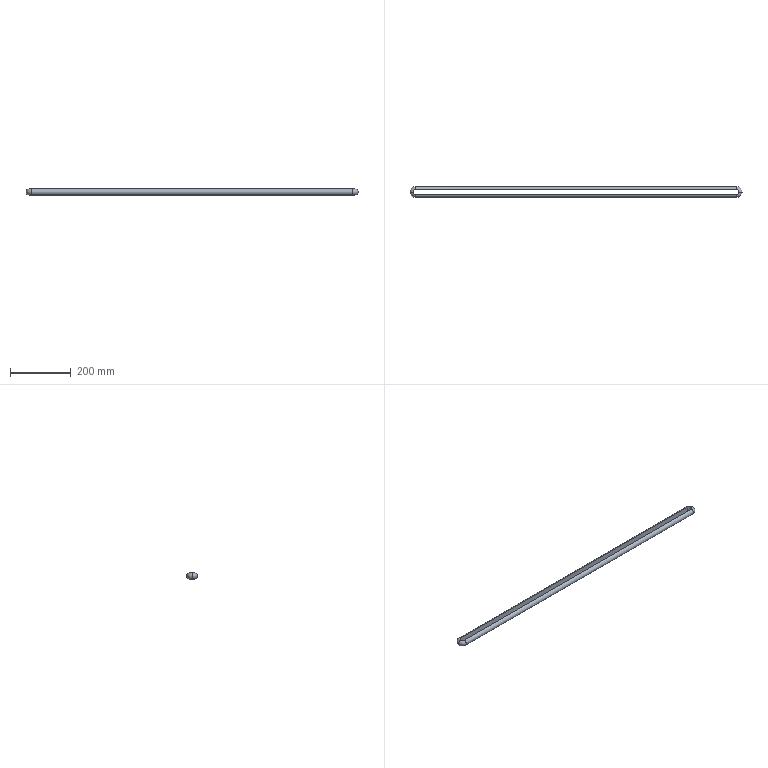Part | SolidWorks | features Sweep 1 | 1 solid | 11 faces | box 1096 x 36 x 20 mm | volume 345093 mm3 | cylinder 5 | torus 4 | plane 2 | commonest cylinder face diameters 16 x3 20 x2
STEP:
#1=CARTESIAN_POINT('',(1060.,8.,10.));
#2=VERTEX_POINT('',#1);
#3=CARTESIAN_POINT('',(1068.,0.,10.));
#4=VERTEX_POINT('',#3);
#5=CARTESIAN_POINT('',(1060.,0.,10.));
#6=DIRECTION('',(0.,0.,-1.));
#7=DIRECTION('',(-1.,0.,0.));
#8=AXIS2_PLACEMENT_3D('',#5,#6,#7);
#9=CIRCLE('',#8,8.);
#10=EDGE_CURVE('',#2,#4,#9,.T.);
#11=ORIENTED_EDGE('',*,*,#10,.T.);
#12=CARTESIAN_POINT('',(1068.,0.,-10.));
#13=VERTEX_POINT('',#12);
#14=CARTESIAN_POINT('',(1068.,0.,0.));
#15=DIRECTION('',(0.,1.,0.));
#16=DIRECTION('',(-1.,0.,0.));
#17=AXIS2_PLACEMENT_3D('',#14,#15,#16);
#18=CIRCLE('',#17,10.);
#19=EDGE_CURVE('',#4,#13,#18,.T.);
#20=ORIENTED_EDGE('',*,*,#19,.T.);
#21=CARTESIAN_POINT('',(1060.,8.,-10.));
#22=VERTEX_POINT('',#21);
#23=CARTESIAN_POINT('',(1060.,0.,-10.));
#24=DIRECTION('',(0.,0.,-1.));
#25=DIRECTION('',(-1.,0.,0.));
#26=AXIS2_PLACEMENT_3D('',#23,#24,#25);
#27=CIRCLE('',#26,8.);
#28=EDGE_CURVE('',#22,#13,#27,.T.);
#29=ORIENTED_EDGE('',*,*,#28,.F.);
#30=CARTESIAN_POINT('',(1060.,8.,0.));
#31=DIRECTION('',(1.,0.,0.));
#32=DIRECTION('',(0.,0.,-1.));
#33=AXIS2_PLACEMENT_3D('',#30,#31,#32);
#34=CIRCLE('',#33,10.);
#35=EDGE_CURVE('',#22,#2,#34,.T.);
#36=ORIENTED_EDGE('',*,*,#35,.T.);
#37=EDGE_LOOP('',(#11,#20,#29,#36));
#38=FACE_OUTER_BOUND('',#37,.T.);
#39=CARTESIAN_POINT('',(1060.,0.,0.));
#40=DIRECTION('',(0.,0.,-1.));
#41=DIRECTION('',(-1.,0.,0.));
#42=AXIS2_PLACEMENT_3D('',#39,#40,#41);
#43=TOROIDAL_SURFACE('',#42,8.,10.);
#44=ADVANCED_FACE('',(#38),#43,.T.);
#45=CARTESIAN_POINT('',(0.,-8.,10.));
#46=VERTEX_POINT('',#45);
#47=CARTESIAN_POINT('',(-8.,0.,10.));
#48=VERTEX_POINT('',#47);
#49=CARTESIAN_POINT('',(0.,0.,10.));
#50=DIRECTION('',(0.,0.,-1.));
#51=DIRECTION('',(-1.,0.,0.));
#52=AXIS2_PLACEMENT_3D('',#49,#50,#51);
#53=CIRCLE('',#52,8.);
#54=EDGE_CURVE('',#46,#48,#53,.T.);
#55=ORIENTED_EDGE('',*,*,#54,.T.);
#56=CARTESIAN_POINT('',(-8.,0.,-10.));
#57=VERTEX_POINT('',#56);
#58=CARTESIAN_POINT('',(-8.,0.,0.));
#59=DIRECTION('',(0.,-1.,0.));
#60=DIRECTION('',(0.,0.,-1.));
#61=AXIS2_PLACEMENT_3D('',#58,#59,#60);
#62=CIRCLE('',#61,10.);
#63=EDGE_CURVE('',#48,#57,#62,.T.);
#64=ORIENTED_EDGE('',*,*,#63,.T.);
#65=CARTESIAN_POINT('',(0.,-8.,-10.));
#66=VERTEX_POINT('',#65);
#67=CARTESIAN_POINT('',(0.,0.,-10.));
#68=DIRECTION('',(0.,0.,-1.));
#69=DIRECTION('',(-1.,0.,0.));
#70=AXIS2_PLACEMENT_3D('',#67,#68,#69);
#71=CIRCLE('',#70,8.);
#72=EDGE_CURVE('',#66,#57,#71,.T.);
#73=ORIENTED_EDGE('',*,*,#72,.F.);
#74=CARTESIAN_POINT('',(0.,-8.,0.));
#75=DIRECTION('',(-1.,0.,0.));
#76=DIRECTION('',(0.,0.,-1.));
#77=AXIS2_PLACEMENT_3D('',#74,#75,#76);
#78=CIRCLE('',#77,10.);
#79=EDGE_CURVE('',#66,#46,#78,.T.);
#80=ORIENTED_EDGE('',*,*,#79,.T.);
#81=EDGE_LOOP('',(#55,#64,#73,#80));
#82=FACE_OUTER_BOUND('',#81,.T.);
#83=CARTESIAN_POINT('',(0.,0.,0.));
#84=DIRECTION('',(0.,0.,-1.));
#85=DIRECTION('',(-1.,0.,0.));
#86=AXIS2_PLACEMENT_3D('',#83,#84,#85);
#87=TOROIDAL_SURFACE('',#86,8.,10.);
#88=ADVANCED_FACE('',(#82),#87,.T.);
#89=CARTESIAN_POINT('',(0.,8.,10.));
#90=VERTEX_POINT('',#89);
#91=CARTESIAN_POINT('',(0.,0.,10.));
#92=DIRECTION('',(0.,0.,-1.));
#93=DIRECTION('',(-1.,0.,0.));
#94=AXIS2_PLACEMENT_3D('',#91,#92,#93);
#95=CIRCLE('',#94,8.);
#96=EDGE_CURVE('',#48,#90,#95,.T.);
#97=ORIENTED_EDGE('',*,*,#96,.F.);
#98=CARTESIAN_POINT('',(-8.,0.,0.));
#99=DIRECTION('',(0.,0.,-1.));
#100=VECTOR('',#99,1000.);
#101=LINE('',#98,#100);
#102=EDGE_CURVE('',#48,#57,#101,.T.);
#103=ORIENTED_EDGE('',*,*,#102,.T.);
#104=CARTESIAN_POINT('',(0.,8.,-10.));
#105=VERTEX_POINT('',#104);
#106=CARTESIAN_POINT('',(0.,0.,-10.));
#107=DIRECTION('',(0.,0.,-1.));
#108=DIRECTION('',(-1.,0.,0.));
#109=AXIS2_PLACEMENT_3D('',#106,#107,#108);
#110=CIRCLE('',#109,8.);
#111=EDGE_CURVE('',#57,#105,#110,.T.);
#112=ORIENTED_EDGE('',*,*,#111,.T.);
#113=CARTESIAN_POINT('',(0.,8.,10.));
#114=CARTESIAN_POINT('',(0.,8.,3.333));
#115=CARTESIAN_POINT('',(0.,8.,-3.333));
#116=CARTESIAN_POINT('',(0.,8.,-10.));
#117=B_SPLINE_CURVE_WITH_KNOTS('',3,(#113,#114,#115,#116),.UNSPECIFIED.,.F.,.F.,(4,4),(0.,1.),.UNSPECIFIED.);
#118=EDGE_CURVE('',#90,#105,#117,.T.);
#119=ORIENTED_EDGE('',*,*,#118,.F.);
#120=EDGE_LOOP('',(#97,#103,#112,#119));
#121=FACE_OUTER_BOUND('',#120,.T.);
#122=CARTESIAN_POINT('',(0.,0.,0.));
#123=DIRECTION('',(0.,0.,-1.));
#124=DIRECTION('',(-1.,0.,0.));
#125=AXIS2_PLACEMENT_3D('',#122,#123,#124);
#126=CYLINDRICAL_SURFACE('',#125,8.);
#127=ADVANCED_FACE('',(#121),#126,.F.);
#128=ORIENTED_EDGE('',*,*,#102,.F.);
#129=ORIENTED_EDGE('',*,*,#54,.F.);
#130=CARTESIAN_POINT('',(0.,-8.,10.));
#131=DIRECTION('',(0.,0.,-1.));
#132=VECTOR('',#131,1000.);
#133=LINE('',#130,#132);
#134=EDGE_CURVE('',#46,#66,#133,.T.);
#135=ORIENTED_EDGE('',*,*,#134,.T.);
#136=ORIENTED_EDGE('',*,*,#72,.T.);
#137=EDGE_LOOP('',(#128,#129,#135,#136));
#138=FACE_OUTER_BOUND('',#137,.T.);
#139=CARTESIAN_POINT('',(0.,0.,0.));
#140=DIRECTION('',(0.,0.,-1.));
#141=DIRECTION('',(-1.,0.,0.));
#142=AXIS2_PLACEMENT_3D('',#139,#140,#141);
#143=CYLINDRICAL_SURFACE('',#142,8.);
#144=ADVANCED_FACE('',(#138),#143,.F.);
#145=ORIENTED_EDGE('',*,*,#63,.F.);
#146=ORIENTED_EDGE('',*,*,#96,.T.);
#147=CARTESIAN_POINT('',(0.,8.,-10.));
#148=CARTESIAN_POINT('',(0.,9.309,-10.));
#149=CARTESIAN_POINT('',(0.,10.617,-9.74));
#150=CARTESIAN_POINT('',(0.,13.036,-8.738));
#151=CARTESIAN_POINT('',(0.,14.145,-7.997));
#152=CARTESIAN_POINT('',(0.,15.997,-6.145));
#153=CARTESIAN_POINT('',(0.,16.738,-5.036));
#154=CARTESIAN_POINT('',(0.,17.74,-2.617));
#155=CARTESIAN_POINT('',(0.,18.,-1.309));
#156=CARTESIAN_POINT('',(0.,18.,1.309));
#157=CARTESIAN_POINT('',(0.,17.74,2.617));
#158=CARTESIAN_POINT('',(0.,16.738,5.036));
#159=CARTESIAN_POINT('',(0.,15.997,6.145));
#160=CARTESIAN_POINT('',(0.,14.145,7.997));
#161=CARTESIAN_POINT('',(0.,13.036,8.738));
#162=CARTESIAN_POINT('',(0.,10.617,9.74));
#163=CARTESIAN_POINT('',(0.,9.309,10.));
#164=CARTESIAN_POINT('',(0.,8.,10.));
#165=B_SPLINE_CURVE_WITH_KNOTS('',3,(#147,#148,#149,#150,#151,#152,#153,#154,#155,#156,#157,#158,#159,#160,#161,#162,#163,#164),.UNSPECIFIED.,.F.,.F.,(4,2,2,2,2,2,2,2,4),(0.,0.125,0.25,0.375,0.5,0.625,0.75,0.875,1.),.UNSPECIFIED.);
#166=EDGE_CURVE('',#105,#90,#165,.T.);
#167=ORIENTED_EDGE('',*,*,#166,.F.);
#168=ORIENTED_EDGE('',*,*,#111,.F.);
#169=EDGE_LOOP('',(#145,#146,#167,#168));
#170=FACE_OUTER_BOUND('',#169,.T.);
#171=CARTESIAN_POINT('',(0.,0.,0.));
#172=DIRECTION('',(0.,0.,-1.));
#173=DIRECTION('',(-1.,0.,0.));
#174=AXIS2_PLACEMENT_3D('',#171,#172,#173);
#175=TOROIDAL_SURFACE('',#174,8.,10.);
#176=ADVANCED_FACE('',(#170),#175,.T.);
#177=CARTESIAN_POINT('',(1060.,-8.,10.));
#178=VERTEX_POINT('',#177);
#179=CARTESIAN_POINT('',(1060.,-8.,-10.));
#180=VERTEX_POINT('',#179);
#181=CARTESIAN_POINT('',(1060.,-8.,10.));
#182=DIRECTION('',(0.,0.,-1.));
#183=VECTOR('',#182,1000.);
#184=LINE('',#181,#183);
#185=EDGE_CURVE('',#178,#180,#184,.T.);
#186=ORIENTED_EDGE('',*,*,#185,.T.);
#187=CARTESIAN_POINT('',(1060.,-8.,-10.));
#188=DIRECTION('',(-1.,0.,0.));
#189=VECTOR('',#188,1000.);
#190=LINE('',#187,#189);
#191=EDGE_CURVE('',#180,#66,#190,.T.);
#192=ORIENTED_EDGE('',*,*,#191,.T.);
#193=ORIENTED_EDGE('',*,*,#134,.F.);
#194=CARTESIAN_POINT('',(1060.,-8.,10.));
#195=DIRECTION('',(-1.,0.,0.));
#196=VECTOR('',#195,1000.);
#197=LINE('',#194,#196);
#198=EDGE_CURVE('',#178,#46,#197,.T.);
#199=ORIENTED_EDGE('',*,*,#198,.F.);
#200=EDGE_LOOP('',(#186,#192,#193,#199));
#201=FACE_OUTER_BOUND('',#200,.T.);
#202=CARTESIAN_POINT('',(1060.,-8.,10.));
#203=DIRECTION('',(0.,1.,0.));
#204=DIRECTION('',(0.,0.,1.));
#205=AXIS2_PLACEMENT_3D('',#202,#203,#204);
#206=PLANE('',#205);
#207=ADVANCED_FACE('',(#201),#206,.T.);
#208=CARTESIAN_POINT('',(1060.,-8.,0.));
#209=DIRECTION('',(-1.,0.,0.));
#210=DIRECTION('',(0.,0.,-1.));
#211=AXIS2_PLACEMENT_3D('',#208,#209,#210);
#212=CIRCLE('',#211,10.);
#213=EDGE_CURVE('',#180,#178,#212,.T.);
#214=ORIENTED_EDGE('',*,*,#213,.T.);
#215=ORIENTED_EDGE('',*,*,#198,.T.);
#216=ORIENTED_EDGE('',*,*,#79,.F.);
#217=ORIENTED_EDGE('',*,*,#191,.F.);
#218=EDGE_LOOP('',(#214,#215,#216,#217));
#219=FACE_OUTER_BOUND('',#218,.T.);
#220=CARTESIAN_POINT('',(1060.,-8.,0.));
#221=DIRECTION('',(-1.,0.,0.));
#222=DIRECTION('',(0.,0.,1.));
#223=AXIS2_PLACEMENT_3D('',#220,#221,#222);
#224=CYLINDRICAL_SURFACE('',#223,10.);
#225=ADVANCED_FACE('',(#219),#224,.T.);
#226=CARTESIAN_POINT('',(1060.,8.,10.));
#227=DIRECTION('',(0.,0.,-1.));
#228=VECTOR('',#227,1000.);
#229=LINE('',#226,#228);
#230=EDGE_CURVE('',#2,#22,#229,.T.);
#231=ORIENTED_EDGE('',*,*,#230,.T.);
#232=ORIENTED_EDGE('',*,*,#28,.T.);
#233=CARTESIAN_POINT('',(1060.,0.,-10.));
#234=DIRECTION('',(0.,0.,-1.));
#235=DIRECTION('',(-1.,0.,0.));
#236=AXIS2_PLACEMENT_3D('',#233,#234,#235);
#237=CIRCLE('',#236,8.);
#238=EDGE_CURVE('',#13,#180,#237,.T.);
#239=ORIENTED_EDGE('',*,*,#238,.T.);
#240=ORIENTED_EDGE('',*,*,#185,.F.);
#241=CARTESIAN_POINT('',(1060.,0.,10.));
#242=DIRECTION('',(0.,0.,-1.));
#243=DIRECTION('',(-1.,0.,0.));
#244=AXIS2_PLACEMENT_3D('',#241,#242,#243);
#245=CIRCLE('',#244,8.);
#246=EDGE_CURVE('',#4,#178,#245,.T.);
#247=ORIENTED_EDGE('',*,*,#246,.F.);
#248=ORIENTED_EDGE('',*,*,#10,.F.);
#249=EDGE_LOOP('',(#231,#232,#239,#240,#247,#248));
#250=FACE_OUTER_BOUND('',#249,.T.);
#251=CARTESIAN_POINT('',(1060.,0.,0.));
#252=DIRECTION('',(0.,0.,-1.));
#253=DIRECTION('',(-1.,0.,0.));
#254=AXIS2_PLACEMENT_3D('',#251,#252,#253);
#255=CYLINDRICAL_SURFACE('',#254,8.);
#256=ADVANCED_FACE('',(#250),#255,.F.);
#257=ORIENTED_EDGE('',*,*,#19,.F.);
#258=ORIENTED_EDGE('',*,*,#246,.T.);
#259=ORIENTED_EDGE('',*,*,#213,.F.);
#260=ORIENTED_EDGE('',*,*,#238,.F.);
#261=EDGE_LOOP('',(#257,#258,#259,#260));
#262=FACE_OUTER_BOUND('',#261,.T.);
#263=CARTESIAN_POINT('',(1060.,0.,0.));
#264=DIRECTION('',(0.,0.,-1.));
#265=DIRECTION('',(-1.,0.,0.));
#266=AXIS2_PLACEMENT_3D('',#263,#264,#265);
#267=TOROIDAL_SURFACE('',#266,8.,10.);
#268=ADVANCED_FACE('',(#262),#267,.T.);
#269=ORIENTED_EDGE('',*,*,#166,.T.);
#270=CARTESIAN_POINT('',(1060.,8.,10.));
#271=DIRECTION('',(-1.,0.,0.));
#272=VECTOR('',#271,1000.);
#273=LINE('',#270,#272);
#274=EDGE_CURVE('',#2,#90,#273,.T.);
#275=ORIENTED_EDGE('',*,*,#274,.F.);
#276=ORIENTED_EDGE('',*,*,#35,.F.);
#277=CARTESIAN_POINT('',(1060.,8.,-10.));
#278=DIRECTION('',(-1.,0.,0.));
#279=VECTOR('',#278,1000.);
#280=LINE('',#277,#279);
#281=EDGE_CURVE('',#22,#105,#280,.T.);
#282=ORIENTED_EDGE('',*,*,#281,.T.);
#283=EDGE_LOOP('',(#269,#275,#276,#282));
#284=FACE_OUTER_BOUND('',#283,.T.);
#285=CARTESIAN_POINT('',(1060.,8.,0.));
#286=DIRECTION('',(-1.,0.,0.));
#287=DIRECTION('',(0.,0.,1.));
#288=AXIS2_PLACEMENT_3D('',#285,#286,#287);
#289=CYLINDRICAL_SURFACE('',#288,10.);
#290=ADVANCED_FACE('',(#284),#289,.T.);
#291=ORIENTED_EDGE('',*,*,#118,.T.);
#292=ORIENTED_EDGE('',*,*,#281,.F.);
#293=ORIENTED_EDGE('',*,*,#230,.F.);
#294=ORIENTED_EDGE('',*,*,#274,.T.);
#295=EDGE_LOOP('',(#291,#292,#293,#294));
#296=FACE_OUTER_BOUND('',#295,.T.);
#297=CARTESIAN_POINT('',(1060.,8.,10.));
#298=DIRECTION('',(0.,1.,0.));
#299=DIRECTION('',(0.,0.,1.));
#300=AXIS2_PLACEMENT_3D('',#297,#298,#299);
#301=PLANE('',#300);
#302=ADVANCED_FACE('',(#296),#301,.F.);
#303=CLOSED_SHELL('',(#44,#88,#127,#144,#176,#207,#225,#256,#268,#290,#302));
#304=MANIFOLD_SOLID_BREP('',#303);
#305=CARTESIAN_POINT('',(0.,0.,0.));
#306=DIRECTION('',(0.,0.,1.));
#307=DIRECTION('',(1.,0.,0.));
#308=AXIS2_PLACEMENT_3D('',#305,#306,#307);
#309=(LENGTH_UNIT()NAMED_UNIT(*)SI_UNIT(.MILLI.,.METRE.));
#310=UNCERTAINTY_MEASURE_WITH_UNIT(LENGTH_MEASURE(0.00001),#309,'','');
#311=(NAMED_UNIT(*)PLANE_ANGLE_UNIT()SI_UNIT($,.RADIAN.));
#312=(NAMED_UNIT(*)SI_UNIT($,.STERADIAN.)SOLID_ANGLE_UNIT());
#313=(GEOMETRIC_REPRESENTATION_CONTEXT(3)GLOBAL_UNCERTAINTY_ASSIGNED_CONTEXT((#310))GLOBAL_UNIT_ASSIGNED_CONTEXT((#309,#311,#312))REPRESENTATION_CONTEXT('',''));
#314=ADVANCED_BREP_SHAPE_REPRESENTATION('',(#304,#308),#313);